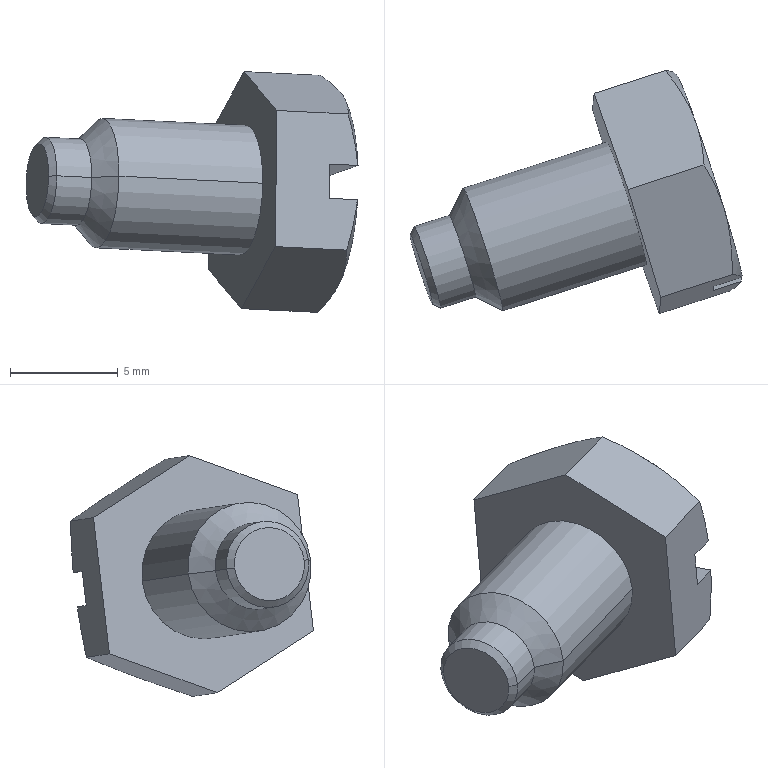Part | SolidWorks | features BaseBody 1 | 1 solid | 27 faces | box 15.373 x 11.248 x 11.146 mm | volume 566.729 mm3 | plane 13 | cone 10 | cylinder 4 | commonest cylinder face diameters 4 x2 6 x2
STEP:
#1=CARTESIAN_POINT('',(72.712,-71.322,-185.285));
#2=VERTEX_POINT('',#1);
#3=CARTESIAN_POINT('',(74.565,-76.993,-184.642));
#4=VERTEX_POINT('',#3);
#5=CARTESIAN_POINT('',(73.639,-74.158,-184.964));
#6=DIRECTION('',(0.9511,0.3055,-0.04654));
#7=DIRECTION('',(0.3088,-0.9451,0.1072));
#8=AXIS2_PLACEMENT_3D('',#5,#6,#7);
#9=CIRCLE('',#8,3.);
#10=EDGE_CURVE('',#2,#4,#9,.T.);
#11=ORIENTED_EDGE('',*,*,#10,.T.);
#12=CARTESIAN_POINT('',(81.223,-74.854,-184.968));
#13=VERTEX_POINT('',#12);
#14=CARTESIAN_POINT('',(73.614,-77.298,-184.596));
#15=DIRECTION('',(0.9511,0.3055,-0.04654));
#16=VECTOR('',#15,1000.);
#17=LINE('',#14,#16);
#18=EDGE_CURVE('',#4,#13,#17,.T.);
#19=ORIENTED_EDGE('',*,*,#18,.T.);
#20=CARTESIAN_POINT('',(79.37,-69.184,-185.611));
#21=VERTEX_POINT('',#20);
#22=CARTESIAN_POINT('',(80.296,-72.019,-185.289));
#23=DIRECTION('',(-0.9511,-0.3055,0.04654));
#24=DIRECTION('',(0.3088,-0.9451,0.1072));
#25=AXIS2_PLACEMENT_3D('',#22,#23,#24);
#26=CIRCLE('',#25,3.);
#27=EDGE_CURVE('',#13,#21,#26,.T.);
#28=ORIENTED_EDGE('',*,*,#27,.T.);
#29=CARTESIAN_POINT('',(71.761,-71.628,-185.239));
#30=DIRECTION('',(0.9511,0.3055,-0.04654));
#31=VECTOR('',#30,1000.);
#32=LINE('',#29,#31);
#33=EDGE_CURVE('',#2,#21,#32,.T.);
#34=ORIENTED_EDGE('',*,*,#33,.F.);
#35=EDGE_LOOP('',(#11,#19,#28,#34));
#36=FACE_OUTER_BOUND('',#35,.T.);
#37=CARTESIAN_POINT('',(72.688,-74.463,-184.917));
#38=DIRECTION('',(0.9511,0.3055,-0.04654));
#39=DIRECTION('',(-0.3088,0.9451,-0.1072));
#40=AXIS2_PLACEMENT_3D('',#37,#38,#39);
#41=CYLINDRICAL_SURFACE('',#40,3.);
#42=ADVANCED_FACE('',(#36),#41,.T.);
#43=CARTESIAN_POINT('',(70.453,-73.092,-185.052));
#44=VERTEX_POINT('',#43);
#45=CARTESIAN_POINT('',(71.689,-76.873,-184.624));
#46=VERTEX_POINT('',#45);
#47=CARTESIAN_POINT('',(71.071,-74.982,-184.838));
#48=DIRECTION('',(0.9511,0.3055,-0.04654));
#49=DIRECTION('',(0.3088,-0.9451,0.1072));
#50=AXIS2_PLACEMENT_3D('',#47,#48,#49);
#51=CIRCLE('',#50,2.);
#52=EDGE_CURVE('',#44,#46,#51,.T.);
#53=ORIENTED_EDGE('',*,*,#52,.T.);
#54=CARTESIAN_POINT('',(73.305,-76.353,-184.703));
#55=VERTEX_POINT('',#54);
#56=CARTESIAN_POINT('',(71.403,-76.964,-184.61));
#57=DIRECTION('',(0.9511,0.3055,-0.04654));
#58=VECTOR('',#57,1000.);
#59=LINE('',#56,#58);
#60=EDGE_CURVE('',#46,#55,#59,.T.);
#61=ORIENTED_EDGE('',*,*,#60,.T.);
#62=CARTESIAN_POINT('',(72.07,-72.573,-185.132));
#63=VERTEX_POINT('',#62);
#64=CARTESIAN_POINT('',(72.688,-74.463,-184.917));
#65=DIRECTION('',(-0.9511,-0.3055,0.04654));
#66=DIRECTION('',(0.3088,-0.9451,0.1072));
#67=AXIS2_PLACEMENT_3D('',#64,#65,#66);
#68=CIRCLE('',#67,2.);
#69=EDGE_CURVE('',#55,#63,#68,.T.);
#70=ORIENTED_EDGE('',*,*,#69,.T.);
#71=CARTESIAN_POINT('',(70.168,-73.184,-185.038));
#72=DIRECTION('',(0.9511,0.3055,-0.04654));
#73=VECTOR('',#72,1000.);
#74=LINE('',#71,#73);
#75=EDGE_CURVE('',#44,#63,#74,.T.);
#76=ORIENTED_EDGE('',*,*,#75,.F.);
#77=EDGE_LOOP('',(#53,#61,#70,#76));
#78=FACE_OUTER_BOUND('',#77,.T.);
#79=CARTESIAN_POINT('',(70.786,-75.074,-184.824));
#80=DIRECTION('',(0.9511,0.3055,-0.04654));
#81=DIRECTION('',(-0.3088,0.9451,-0.1072));
#82=AXIS2_PLACEMENT_3D('',#79,#80,#81);
#83=CYLINDRICAL_SURFACE('',#82,2.);
#84=ADVANCED_FACE('',(#78),#83,.T.);
#85=CARTESIAN_POINT('',(71.311,-76.681,-184.642));
#86=VERTEX_POINT('',#85);
#87=CARTESIAN_POINT('',(70.261,-73.467,-185.006));
#88=VERTEX_POINT('',#87);
#89=CARTESIAN_POINT('',(70.786,-75.074,-184.824));
#90=DIRECTION('',(-0.9511,-0.3055,0.04654));
#91=DIRECTION('',(0.3088,-0.9451,0.1072));
#92=AXIS2_PLACEMENT_3D('',#89,#90,#91);
#93=CIRCLE('',#92,1.7);
#94=EDGE_CURVE('',#86,#88,#93,.T.);
#95=ORIENTED_EDGE('',*,*,#94,.F.);
#96=CARTESIAN_POINT('',(71.311,-76.681,-184.642));
#97=DIRECTION('',(0.8909,-0.4522,0.04287));
#98=VECTOR('',#97,1000.);
#99=LINE('',#96,#98);
#100=EDGE_CURVE('',#86,#46,#99,.T.);
#101=ORIENTED_EDGE('',*,*,#100,.T.);
#102=ORIENTED_EDGE('',*,*,#52,.F.);
#103=CARTESIAN_POINT('',(70.261,-73.467,-185.006));
#104=DIRECTION('',(0.4541,0.8843,-0.1087));
#105=VECTOR('',#104,1000.);
#106=LINE('',#103,#105);
#107=EDGE_CURVE('',#88,#44,#106,.T.);
#108=ORIENTED_EDGE('',*,*,#107,.F.);
#109=EDGE_LOOP('',(#95,#101,#102,#108));
#110=FACE_OUTER_BOUND('',#109,.T.);
#111=CARTESIAN_POINT('',(70.786,-75.074,-184.824));
#112=DIRECTION('',(0.9511,0.3055,-0.04654));
#113=DIRECTION('',(-0.3088,0.9451,-0.1072));
#114=AXIS2_PLACEMENT_3D('',#111,#112,#113);
#115=CONICAL_SURFACE('',#114,1.7,0.7854);
#116=ADVANCED_FACE('',(#110),#115,.T.);
#117=ORIENTED_EDGE('',*,*,#69,.F.);
#118=CARTESIAN_POINT('',(73.305,-76.353,-184.703));
#119=DIRECTION('',(0.8909,-0.4522,0.04287));
#120=VECTOR('',#119,1000.);
#121=LINE('',#118,#120);
#122=EDGE_CURVE('',#55,#4,#121,.T.);
#123=ORIENTED_EDGE('',*,*,#122,.T.);
#124=ORIENTED_EDGE('',*,*,#10,.F.);
#125=CARTESIAN_POINT('',(72.07,-72.573,-185.132));
#126=DIRECTION('',(0.4541,0.8843,-0.1087));
#127=VECTOR('',#126,1000.);
#128=LINE('',#125,#127);
#129=EDGE_CURVE('',#63,#2,#128,.T.);
#130=ORIENTED_EDGE('',*,*,#129,.F.);
#131=EDGE_LOOP('',(#117,#123,#124,#130));
#132=FACE_OUTER_BOUND('',#131,.T.);
#133=CARTESIAN_POINT('',(72.688,-74.463,-184.917));
#134=DIRECTION('',(0.9511,0.3055,-0.04654));
#135=DIRECTION('',(-0.3088,0.9451,-0.1072));
#136=AXIS2_PLACEMENT_3D('',#133,#134,#135);
#137=CONICAL_SURFACE('',#136,2.,0.7854);
#138=ADVANCED_FACE('',(#132),#137,.T.);
#139=CARTESIAN_POINT('',(84.322,-75.857,-184.08));
#140=VERTEX_POINT('',#139);
#141=CARTESIAN_POINT('',(84.304,-76.043,-185.669));
#142=VERTEX_POINT('',#141);
#143=CARTESIAN_POINT('',(84.322,-75.857,-184.08));
#144=DIRECTION('',(-0.01125,-0.1163,-0.9932));
#145=VECTOR('',#144,1000.);
#146=LINE('',#143,#145);
#147=EDGE_CURVE('',#140,#142,#146,.T.);
#148=ORIENTED_EDGE('',*,*,#147,.T.);
#149=CARTESIAN_POINT('',(81.216,-66.593,-186.741));
#150=VERTEX_POINT('',#149);
#151=CARTESIAN_POINT('',(84.304,-76.043,-185.669));
#152=DIRECTION('',(-0.3088,0.9451,-0.1072));
#153=VECTOR('',#152,1000.);
#154=LINE('',#151,#153);
#155=EDGE_CURVE('',#142,#150,#154,.T.);
#156=ORIENTED_EDGE('',*,*,#155,.T.);
#157=CARTESIAN_POINT('',(81.234,-66.407,-185.152));
#158=VERTEX_POINT('',#157);
#159=CARTESIAN_POINT('',(81.216,-66.593,-186.741));
#160=DIRECTION('',(0.01125,0.1163,0.9932));
#161=VECTOR('',#160,1000.);
#162=LINE('',#159,#161);
#163=EDGE_CURVE('',#150,#158,#162,.T.);
#164=ORIENTED_EDGE('',*,*,#163,.T.);
#165=CARTESIAN_POINT('',(84.322,-75.857,-184.08));
#166=DIRECTION('',(0.3088,-0.9451,0.1072));
#167=VECTOR('',#166,1000.);
#168=LINE('',#165,#167);
#169=EDGE_CURVE('',#158,#140,#168,.T.);
#170=ORIENTED_EDGE('',*,*,#169,.T.);
#171=EDGE_LOOP('',(#148,#156,#164,#170));
#172=FACE_OUTER_BOUND('',#171,.T.);
#173=CARTESIAN_POINT('',(84.304,-76.043,-185.669));
#174=DIRECTION('',(0.9511,0.3055,-0.04654));
#175=DIRECTION('',(0.,-0.1506,-0.9886));
#176=AXIS2_PLACEMENT_3D('',#173,#174,#175);
#177=PLANE('',#176);
#178=ADVANCED_FACE('',(#172),#177,.T.);
#179=CARTESIAN_POINT('',(82.567,-66.226,-186.799));
#180=VERTEX_POINT('',#179);
#181=CARTESIAN_POINT('',(82.512,-66.176,-186.804));
#182=VERTEX_POINT('',#181);
#183=CARTESIAN_POINT('',(82.567,-66.226,-186.799));
#184=CARTESIAN_POINT('',(82.549,-66.209,-186.801));
#185=CARTESIAN_POINT('',(82.531,-66.193,-186.803));
#186=CARTESIAN_POINT('',(82.512,-66.176,-186.804));
#187=B_SPLINE_CURVE_WITH_KNOTS('',3,(#183,#184,#185,#186),.UNSPECIFIED.,.F.,.F.,(4,4),(0.,1.),.UNSPECIFIED.);
#188=EDGE_CURVE('',#180,#182,#187,.T.);
#189=ORIENTED_EDGE('',*,*,#188,.T.);
#190=CARTESIAN_POINT('',(81.216,-66.593,-186.741));
#191=DIRECTION('',(0.9511,0.3055,-0.04654));
#192=VECTOR('',#191,1000.);
#193=LINE('',#190,#192);
#194=EDGE_CURVE('',#150,#182,#193,.T.);
#195=ORIENTED_EDGE('',*,*,#194,.F.);
#196=ORIENTED_EDGE('',*,*,#155,.F.);
#197=CARTESIAN_POINT('',(85.601,-75.627,-185.733));
#198=VERTEX_POINT('',#197);
#199=CARTESIAN_POINT('',(84.304,-76.043,-185.669));
#200=DIRECTION('',(0.9511,0.3055,-0.04654));
#201=VECTOR('',#200,1000.);
#202=LINE('',#199,#201);
#203=EDGE_CURVE('',#142,#198,#202,.T.);
#204=ORIENTED_EDGE('',*,*,#203,.T.);
#205=CARTESIAN_POINT('',(85.616,-75.555,-185.741));
#206=VERTEX_POINT('',#205);
#207=CARTESIAN_POINT('',(85.601,-75.627,-185.733));
#208=CARTESIAN_POINT('',(85.605,-75.605,-185.735));
#209=CARTESIAN_POINT('',(85.61,-75.582,-185.738));
#210=CARTESIAN_POINT('',(85.615,-75.558,-185.741));
#211=CARTESIAN_POINT('',(85.615,-75.557,-185.741));
#212=CARTESIAN_POINT('',(85.616,-75.555,-185.741));
#213=B_SPLINE_CURVE_WITH_KNOTS('',3,(#207,#208,#209,#210,#211,#212),.UNSPECIFIED.,.F.,.F.,(4,2,4),(0.,0.9225,1.),.UNSPECIFIED.);
#214=EDGE_CURVE('',#198,#206,#213,.T.);
#215=ORIENTED_EDGE('',*,*,#214,.T.);
#216=CARTESIAN_POINT('',(85.635,-75.616,-185.734));
#217=DIRECTION('',(-0.3088,0.9451,-0.1072));
#218=VECTOR('',#217,1000.);
#219=LINE('',#216,#218);
#220=EDGE_CURVE('',#206,#180,#219,.T.);
#221=ORIENTED_EDGE('',*,*,#220,.T.);
#222=EDGE_LOOP('',(#189,#195,#196,#204,#215,#221));
#223=FACE_OUTER_BOUND('',#222,.T.);
#224=CARTESIAN_POINT('',(84.304,-76.043,-185.669));
#225=DIRECTION('',(-0.01125,-0.1163,-0.9932));
#226=DIRECTION('',(0.,-0.9932,0.1163));
#227=AXIS2_PLACEMENT_3D('',#224,#225,#226);
#228=PLANE('',#227);
#229=ADVANCED_FACE('',(#223),#228,.F.);
#230=CARTESIAN_POINT('',(85.634,-75.369,-184.152));
#231=VERTEX_POINT('',#230);
#232=CARTESIAN_POINT('',(85.619,-75.441,-184.144));
#233=VERTEX_POINT('',#232);
#234=CARTESIAN_POINT('',(85.634,-75.369,-184.152));
#235=CARTESIAN_POINT('',(85.629,-75.393,-184.149));
#236=CARTESIAN_POINT('',(85.624,-75.417,-184.146));
#237=CARTESIAN_POINT('',(85.619,-75.441,-184.144));
#238=B_SPLINE_CURVE_WITH_KNOTS('',3,(#234,#235,#236,#237),.UNSPECIFIED.,.F.,.F.,(4,4),(0.,1.),.UNSPECIFIED.);
#239=EDGE_CURVE('',#231,#233,#238,.T.);
#240=ORIENTED_EDGE('',*,*,#239,.T.);
#241=CARTESIAN_POINT('',(84.322,-75.857,-184.08));
#242=DIRECTION('',(0.9511,0.3055,-0.04654));
#243=VECTOR('',#242,1000.);
#244=LINE('',#241,#243);
#245=EDGE_CURVE('',#140,#233,#244,.T.);
#246=ORIENTED_EDGE('',*,*,#245,.F.);
#247=ORIENTED_EDGE('',*,*,#169,.F.);
#248=CARTESIAN_POINT('',(82.53,-65.99,-185.215));
#249=VERTEX_POINT('',#248);
#250=CARTESIAN_POINT('',(81.234,-66.407,-185.152));
#251=DIRECTION('',(0.9511,0.3055,-0.04654));
#252=VECTOR('',#251,1000.);
#253=LINE('',#250,#252);
#254=EDGE_CURVE('',#158,#249,#253,.T.);
#255=ORIENTED_EDGE('',*,*,#254,.T.);
#256=CARTESIAN_POINT('',(82.585,-66.04,-185.21));
#257=VERTEX_POINT('',#256);
#258=CARTESIAN_POINT('',(82.53,-65.99,-185.215));
#259=CARTESIAN_POINT('',(82.547,-66.005,-185.214));
#260=CARTESIAN_POINT('',(82.564,-66.021,-185.212));
#261=CARTESIAN_POINT('',(82.582,-66.037,-185.21));
#262=CARTESIAN_POINT('',(82.584,-66.038,-185.21));
#263=CARTESIAN_POINT('',(82.585,-66.04,-185.21));
#264=B_SPLINE_CURVE_WITH_KNOTS('',3,(#258,#259,#260,#261,#262,#263),.UNSPECIFIED.,.F.,.F.,(4,2,4),(0.,0.9225,1.),.UNSPECIFIED.);
#265=EDGE_CURVE('',#249,#257,#264,.T.);
#266=ORIENTED_EDGE('',*,*,#265,.T.);
#267=CARTESIAN_POINT('',(85.653,-75.43,-184.145));
#268=DIRECTION('',(0.3088,-0.9451,0.1072));
#269=VECTOR('',#268,1000.);
#270=LINE('',#267,#269);
#271=EDGE_CURVE('',#257,#231,#270,.T.);
#272=ORIENTED_EDGE('',*,*,#271,.T.);
#273=EDGE_LOOP('',(#240,#246,#247,#255,#266,#272));
#274=FACE_OUTER_BOUND('',#273,.T.);
#275=CARTESIAN_POINT('',(84.322,-75.857,-184.08));
#276=DIRECTION('',(0.01125,0.1163,0.9932));
#277=DIRECTION('',(0.9954,-0.09625,0.));
#278=AXIS2_PLACEMENT_3D('',#275,#276,#277);
#279=PLANE('',#278);
#280=ADVANCED_FACE('',(#274),#279,.F.);
#281=ORIENTED_EDGE('',*,*,#220,.F.);
#282=CARTESIAN_POINT('',(84.706,-73.334,-189.742));
#283=VERTEX_POINT('',#282);
#284=CARTESIAN_POINT('',(84.1,-70.797,-185.476));
#285=DIRECTION('',(0.9511,0.3055,-0.04654));
#286=DIRECTION('',(-0.3088,0.9451,-0.1072));
#287=AXIS2_PLACEMENT_3D('',#284,#285,#286);
#288=CIRCLE('',#287,5.);
#289=EDGE_CURVE('',#206,#283,#288,.T.);
#290=ORIENTED_EDGE('',*,*,#289,.T.);
#291=CARTESIAN_POINT('',(83.393,-69.313,-190.198));
#292=VERTEX_POINT('',#291);
#293=CARTESIAN_POINT('',(84.1,-70.797,-185.476));
#294=DIRECTION('',(0.9511,0.3055,-0.04654));
#295=DIRECTION('',(-0.3088,0.9451,-0.1072));
#296=AXIS2_PLACEMENT_3D('',#293,#294,#295);
#297=CIRCLE('',#296,5.);
#298=EDGE_CURVE('',#283,#292,#297,.T.);
#299=ORIENTED_EDGE('',*,*,#298,.T.);
#300=CARTESIAN_POINT('',(84.1,-70.797,-185.476));
#301=DIRECTION('',(0.9511,0.3055,-0.04654));
#302=DIRECTION('',(-0.3088,0.9451,-0.1072));
#303=AXIS2_PLACEMENT_3D('',#300,#301,#302);
#304=CIRCLE('',#303,5.);
#305=EDGE_CURVE('',#292,#180,#304,.T.);
#306=ORIENTED_EDGE('',*,*,#305,.T.);
#307=EDGE_LOOP('',(#281,#290,#299,#306));
#308=FACE_OUTER_BOUND('',#307,.T.);
#309=CARTESIAN_POINT('',(82.592,-65.703,-182.859));
#310=DIRECTION('',(0.9511,0.3055,-0.04654));
#311=DIRECTION('',(0.,-0.1506,-0.9886));
#312=AXIS2_PLACEMENT_3D('',#309,#310,#311);
#313=PLANE('',#312);
#314=ADVANCED_FACE('',(#308),#313,.T.);
#315=ORIENTED_EDGE('',*,*,#265,.F.);
#316=CARTESIAN_POINT('',(82.085,-65.865,-182.834));
#317=VERTEX_POINT('',#316);
#318=CARTESIAN_POINT('',(82.53,-65.99,-185.215));
#319=CARTESIAN_POINT('',(82.469,-65.918,-184.407));
#320=CARTESIAN_POINT('',(82.305,-65.882,-183.616));
#321=CARTESIAN_POINT('',(82.085,-65.865,-182.834));
#322=B_SPLINE_CURVE_WITH_KNOTS('',3,(#318,#319,#320,#321),.UNSPECIFIED.,.F.,.F.,(4,4),(0.,0.002426),.UNSPECIFIED.);
#323=EDGE_CURVE('',#249,#317,#322,.T.);
#324=ORIENTED_EDGE('',*,*,#323,.T.);
#325=CARTESIAN_POINT('',(83.494,-68.261,-181.21));
#326=VERTEX_POINT('',#325);
#327=CARTESIAN_POINT('',(82.085,-65.865,-182.834));
#328=CARTESIAN_POINT('',(82.684,-66.601,-182.312));
#329=CARTESIAN_POINT('',(83.185,-67.384,-181.775));
#330=CARTESIAN_POINT('',(83.494,-68.261,-181.21));
#331=B_SPLINE_CURVE_WITH_KNOTS('',3,(#327,#328,#329,#330),.UNSPECIFIED.,.F.,.F.,(4,4),(0.,0.003219),.UNSPECIFIED.);
#332=EDGE_CURVE('',#317,#326,#331,.T.);
#333=ORIENTED_EDGE('',*,*,#332,.T.);
#334=CARTESIAN_POINT('',(84.1,-70.797,-185.476));
#335=DIRECTION('',(0.9511,0.3055,-0.04654));
#336=DIRECTION('',(-0.3088,0.9451,-0.1072));
#337=AXIS2_PLACEMENT_3D('',#334,#335,#336);
#338=CIRCLE('',#337,5.);
#339=EDGE_CURVE('',#257,#326,#338,.T.);
#340=ORIENTED_EDGE('',*,*,#339,.F.);
#341=EDGE_LOOP('',(#315,#324,#333,#340));
#342=FACE_OUTER_BOUND('',#341,.T.);
#343=CARTESIAN_POINT('',(84.1,-70.797,-185.476));
#344=DIRECTION('',(-0.9511,-0.3055,0.04654));
#345=DIRECTION('',(-0.3088,0.9451,-0.1072));
#346=AXIS2_PLACEMENT_3D('',#343,#344,#345);
#347=CONICAL_SURFACE('',#346,5.,1.047);
#348=ADVANCED_FACE('',(#342),#347,.T.);
#349=CARTESIAN_POINT('',(83.874,-70.247,-179.974));
#350=VERTEX_POINT('',#349);
#351=CARTESIAN_POINT('',(83.494,-68.261,-181.21));
#352=CARTESIAN_POINT('',(83.721,-68.902,-180.796));
#353=CARTESIAN_POINT('',(83.835,-69.567,-180.384));
#354=CARTESIAN_POINT('',(83.874,-70.247,-179.974));
#355=B_SPLINE_CURVE_WITH_KNOTS('',3,(#351,#352,#353,#354),.UNSPECIFIED.,.F.,.F.,(4,4),(0.,0.00237),.UNSPECIFIED.);
#356=EDGE_CURVE('',#326,#350,#355,.T.);
#357=ORIENTED_EDGE('',*,*,#356,.T.);
#358=CARTESIAN_POINT('',(84.808,-72.281,-180.754));
#359=VERTEX_POINT('',#358);
#360=CARTESIAN_POINT('',(83.874,-70.247,-179.974));
#361=CARTESIAN_POINT('',(84.267,-70.888,-180.235));
#362=CARTESIAN_POINT('',(84.589,-71.561,-180.494));
#363=CARTESIAN_POINT('',(84.808,-72.281,-180.754));
#364=B_SPLINE_CURVE_WITH_KNOTS('',3,(#360,#361,#362,#363),.UNSPECIFIED.,.F.,.F.,(4,4),(0.,0.00237),.UNSPECIFIED.);
#365=EDGE_CURVE('',#350,#359,#364,.T.);
#366=ORIENTED_EDGE('',*,*,#365,.T.);
#367=CARTESIAN_POINT('',(84.1,-70.797,-185.476));
#368=DIRECTION('',(0.9511,0.3055,-0.04654));
#369=DIRECTION('',(-0.3088,0.9451,-0.1072));
#370=AXIS2_PLACEMENT_3D('',#367,#368,#369);
#371=CIRCLE('',#370,5.);
#372=EDGE_CURVE('',#326,#359,#371,.T.);
#373=ORIENTED_EDGE('',*,*,#372,.F.);
#374=EDGE_LOOP('',(#357,#366,#373));
#375=FACE_OUTER_BOUND('',#374,.T.);
#376=CARTESIAN_POINT('',(84.1,-70.797,-185.476));
#377=DIRECTION('',(-0.9511,-0.3055,0.04654));
#378=DIRECTION('',(-0.3088,0.9451,-0.1072));
#379=AXIS2_PLACEMENT_3D('',#376,#377,#378);
#380=CONICAL_SURFACE('',#379,5.,1.047);
#381=ADVANCED_FACE('',(#375),#380,.T.);
#382=ORIENTED_EDGE('',*,*,#239,.F.);
#383=CARTESIAN_POINT('',(84.1,-70.797,-185.476));
#384=DIRECTION('',(0.9511,0.3055,-0.04654));
#385=DIRECTION('',(-0.3088,0.9451,-0.1072));
#386=AXIS2_PLACEMENT_3D('',#383,#384,#385);
#387=CIRCLE('',#386,5.);
#388=EDGE_CURVE('',#359,#231,#387,.T.);
#389=ORIENTED_EDGE('',*,*,#388,.F.);
#390=CARTESIAN_POINT('',(85.174,-75.316,-181.762));
#391=VERTEX_POINT('',#390);
#392=CARTESIAN_POINT('',(84.808,-72.281,-180.754));
#393=CARTESIAN_POINT('',(85.107,-73.266,-181.108));
#394=CARTESIAN_POINT('',(85.194,-74.283,-181.441));
#395=CARTESIAN_POINT('',(85.174,-75.316,-181.762));
#396=B_SPLINE_CURVE_WITH_KNOTS('',3,(#392,#393,#394,#395),.UNSPECIFIED.,.F.,.F.,(4,4),(0.,0.003219),.UNSPECIFIED.);
#397=EDGE_CURVE('',#359,#391,#396,.T.);
#398=ORIENTED_EDGE('',*,*,#397,.T.);
#399=CARTESIAN_POINT('',(85.174,-75.316,-181.762));
#400=CARTESIAN_POINT('',(85.393,-75.333,-182.544));
#401=CARTESIAN_POINT('',(85.557,-75.369,-183.335));
#402=CARTESIAN_POINT('',(85.619,-75.441,-184.144));
#403=B_SPLINE_CURVE_WITH_KNOTS('',3,(#399,#400,#401,#402),.UNSPECIFIED.,.F.,.F.,(4,4),(0.,0.002426),.UNSPECIFIED.);
#404=EDGE_CURVE('',#391,#233,#403,.T.);
#405=ORIENTED_EDGE('',*,*,#404,.T.);
#406=EDGE_LOOP('',(#382,#389,#398,#405));
#407=FACE_OUTER_BOUND('',#406,.T.);
#408=CARTESIAN_POINT('',(84.1,-70.797,-185.476));
#409=DIRECTION('',(-0.9511,-0.3055,0.04654));
#410=DIRECTION('',(-0.3088,0.9451,-0.1072));
#411=AXIS2_PLACEMENT_3D('',#408,#409,#410);
#412=CONICAL_SURFACE('',#411,5.,1.047);
#413=ADVANCED_FACE('',(#407),#412,.T.);
#414=ORIENTED_EDGE('',*,*,#214,.F.);
#415=CARTESIAN_POINT('',(85.102,-76.054,-188.068));
#416=VERTEX_POINT('',#415);
#417=CARTESIAN_POINT('',(85.601,-75.627,-185.733));
#418=CARTESIAN_POINT('',(85.521,-75.744,-186.534));
#419=CARTESIAN_POINT('',(85.339,-75.891,-187.308));
#420=CARTESIAN_POINT('',(85.102,-76.054,-188.068));
#421=B_SPLINE_CURVE_WITH_KNOTS('',3,(#417,#418,#419,#420),.UNSPECIFIED.,.F.,.F.,(4,4),(0.,0.002426),.UNSPECIFIED.);
#422=EDGE_CURVE('',#198,#416,#421,.T.);
#423=ORIENTED_EDGE('',*,*,#422,.T.);
#424=CARTESIAN_POINT('',(85.102,-76.054,-188.068));
#425=CARTESIAN_POINT('',(85.113,-75.123,-188.62));
#426=CARTESIAN_POINT('',(85.016,-74.21,-189.176));
#427=CARTESIAN_POINT('',(84.706,-73.334,-189.742));
#428=B_SPLINE_CURVE_WITH_KNOTS('',3,(#424,#425,#426,#427),.UNSPECIFIED.,.F.,.F.,(4,4),(0.,0.003219),.UNSPECIFIED.);
#429=EDGE_CURVE('',#416,#283,#428,.T.);
#430=ORIENTED_EDGE('',*,*,#429,.T.);
#431=ORIENTED_EDGE('',*,*,#289,.F.);
#432=EDGE_LOOP('',(#414,#423,#430,#431));
#433=FACE_OUTER_BOUND('',#432,.T.);
#434=CARTESIAN_POINT('',(84.1,-70.797,-185.476));
#435=DIRECTION('',(-0.9511,-0.3055,0.04654));
#436=DIRECTION('',(-0.3088,0.9451,-0.1072));
#437=AXIS2_PLACEMENT_3D('',#434,#435,#436);
#438=CONICAL_SURFACE('',#437,5.,1.047);
#439=ADVANCED_FACE('',(#433),#438,.T.);
#440=CARTESIAN_POINT('',(83.75,-71.532,-190.949));
#441=VERTEX_POINT('',#440);
#442=CARTESIAN_POINT('',(83.75,-71.532,-190.949));
#443=CARTESIAN_POINT('',(83.718,-70.776,-190.706));
#444=CARTESIAN_POINT('',(83.611,-70.034,-190.457));
#445=CARTESIAN_POINT('',(83.393,-69.313,-190.198));
#446=B_SPLINE_CURVE_WITH_KNOTS('',3,(#442,#443,#444,#445),.UNSPECIFIED.,.F.,.F.,(4,4),(0.,0.00237),.UNSPECIFIED.);
#447=EDGE_CURVE('',#441,#292,#446,.T.);
#448=ORIENTED_EDGE('',*,*,#447,.T.);
#449=ORIENTED_EDGE('',*,*,#298,.F.);
#450=CARTESIAN_POINT('',(84.706,-73.334,-189.742));
#451=CARTESIAN_POINT('',(84.48,-72.692,-190.155));
#452=CARTESIAN_POINT('',(84.15,-72.097,-190.556));
#453=CARTESIAN_POINT('',(83.75,-71.532,-190.949));
#454=B_SPLINE_CURVE_WITH_KNOTS('',3,(#450,#451,#452,#453),.UNSPECIFIED.,.F.,.F.,(4,4),(0.,0.00237),.UNSPECIFIED.);
#455=EDGE_CURVE('',#283,#441,#454,.T.);
#456=ORIENTED_EDGE('',*,*,#455,.T.);
#457=EDGE_LOOP('',(#448,#449,#456));
#458=FACE_OUTER_BOUND('',#457,.T.);
#459=CARTESIAN_POINT('',(84.1,-70.797,-185.476));
#460=DIRECTION('',(-0.9511,-0.3055,0.04654));
#461=DIRECTION('',(-0.3088,0.9451,-0.1072));
#462=AXIS2_PLACEMENT_3D('',#459,#460,#461);
#463=CONICAL_SURFACE('',#462,5.,1.047);
#464=ADVANCED_FACE('',(#458),#463,.T.);
#465=ORIENTED_EDGE('',*,*,#188,.F.);
#466=ORIENTED_EDGE('',*,*,#305,.F.);
#467=CARTESIAN_POINT('',(82.014,-66.604,-189.139));
#468=VERTEX_POINT('',#467);
#469=CARTESIAN_POINT('',(83.393,-69.313,-190.198));
#470=CARTESIAN_POINT('',(83.094,-68.329,-189.843));
#471=CARTESIAN_POINT('',(82.603,-67.442,-189.491));
#472=CARTESIAN_POINT('',(82.014,-66.604,-189.139));
#473=B_SPLINE_CURVE_WITH_KNOTS('',3,(#469,#470,#471,#472),.UNSPECIFIED.,.F.,.F.,(4,4),(0.,0.003219),.UNSPECIFIED.);
#474=EDGE_CURVE('',#292,#468,#473,.T.);
#475=ORIENTED_EDGE('',*,*,#474,.T.);
#476=CARTESIAN_POINT('',(82.014,-66.604,-189.139));
#477=CARTESIAN_POINT('',(82.251,-66.44,-188.38));
#478=CARTESIAN_POINT('',(82.433,-66.293,-187.606));
#479=CARTESIAN_POINT('',(82.512,-66.176,-186.804));
#480=B_SPLINE_CURVE_WITH_KNOTS('',3,(#476,#477,#478,#479),.UNSPECIFIED.,.F.,.F.,(4,4),(0.,0.002426),.UNSPECIFIED.);
#481=EDGE_CURVE('',#468,#182,#480,.T.);
#482=ORIENTED_EDGE('',*,*,#481,.T.);
#483=EDGE_LOOP('',(#465,#466,#475,#482));
#484=FACE_OUTER_BOUND('',#483,.T.);
#485=CARTESIAN_POINT('',(84.1,-70.797,-185.476));
#486=DIRECTION('',(-0.9511,-0.3055,0.04654));
#487=DIRECTION('',(-0.3088,0.9451,-0.1072));
#488=AXIS2_PLACEMENT_3D('',#485,#486,#487);
#489=CONICAL_SURFACE('',#488,5.,1.047);
#490=ADVANCED_FACE('',(#484),#489,.T.);
#491=ORIENTED_EDGE('',*,*,#122,.F.);
#492=CARTESIAN_POINT('',(72.688,-74.463,-184.917));
#493=DIRECTION('',(-0.9511,-0.3055,0.04654));
#494=DIRECTION('',(0.3088,-0.9451,0.1072));
#495=AXIS2_PLACEMENT_3D('',#492,#493,#494);
#496=CIRCLE('',#495,2.);
#497=EDGE_CURVE('',#63,#55,#496,.T.);
#498=ORIENTED_EDGE('',*,*,#497,.F.);
#499=ORIENTED_EDGE('',*,*,#129,.T.);
#500=CARTESIAN_POINT('',(73.639,-74.158,-184.964));
#501=DIRECTION('',(0.9511,0.3055,-0.04654));
#502=DIRECTION('',(0.3088,-0.9451,0.1072));
#503=AXIS2_PLACEMENT_3D('',#500,#501,#502);
#504=CIRCLE('',#503,3.);
#505=EDGE_CURVE('',#4,#2,#504,.T.);
#506=ORIENTED_EDGE('',*,*,#505,.F.);
#507=EDGE_LOOP('',(#491,#498,#499,#506));
#508=FACE_OUTER_BOUND('',#507,.T.);
#509=CARTESIAN_POINT('',(72.688,-74.463,-184.917));
#510=DIRECTION('',(0.9511,0.3055,-0.04654));
#511=DIRECTION('',(-0.3088,0.9451,-0.1072));
#512=AXIS2_PLACEMENT_3D('',#509,#510,#511);
#513=CONICAL_SURFACE('',#512,2.,0.7854);
#514=ADVANCED_FACE('',(#508),#513,.T.);
#515=ORIENTED_EDGE('',*,*,#100,.F.);
#516=CARTESIAN_POINT('',(70.786,-75.074,-184.824));
#517=DIRECTION('',(-0.9511,-0.3055,0.04654));
#518=DIRECTION('',(0.3088,-0.9451,0.1072));
#519=AXIS2_PLACEMENT_3D('',#516,#517,#518);
#520=CIRCLE('',#519,1.7);
#521=EDGE_CURVE('',#88,#86,#520,.T.);
#522=ORIENTED_EDGE('',*,*,#521,.F.);
#523=ORIENTED_EDGE('',*,*,#107,.T.);
#524=CARTESIAN_POINT('',(71.071,-74.982,-184.838));
#525=DIRECTION('',(0.9511,0.3055,-0.04654));
#526=DIRECTION('',(0.3088,-0.9451,0.1072));
#527=AXIS2_PLACEMENT_3D('',#524,#525,#526);
#528=CIRCLE('',#527,2.);
#529=EDGE_CURVE('',#46,#44,#528,.T.);
#530=ORIENTED_EDGE('',*,*,#529,.F.);
#531=EDGE_LOOP('',(#515,#522,#523,#530));
#532=FACE_OUTER_BOUND('',#531,.T.);
#533=CARTESIAN_POINT('',(70.786,-75.074,-184.824));
#534=DIRECTION('',(0.9511,0.3055,-0.04654));
#535=DIRECTION('',(-0.3088,0.9451,-0.1072));
#536=AXIS2_PLACEMENT_3D('',#533,#534,#535);
#537=CONICAL_SURFACE('',#536,1.7,0.7854);
#538=ADVANCED_FACE('',(#532),#537,.T.);
#539=ORIENTED_EDGE('',*,*,#521,.T.);
#540=ORIENTED_EDGE('',*,*,#94,.T.);
#541=EDGE_LOOP('',(#539,#540));
#542=FACE_OUTER_BOUND('',#541,.T.);
#543=CARTESIAN_POINT('',(70.786,-75.074,-184.824));
#544=DIRECTION('',(-0.9511,-0.3055,0.04654));
#545=DIRECTION('',(-0.3058,0.9521,0.));
#546=AXIS2_PLACEMENT_3D('',#543,#544,#545);
#547=PLANE('',#546);
#548=ADVANCED_FACE('',(#542),#547,.T.);
#549=ORIENTED_EDGE('',*,*,#60,.F.);
#550=ORIENTED_EDGE('',*,*,#529,.T.);
#551=ORIENTED_EDGE('',*,*,#75,.T.);
#552=ORIENTED_EDGE('',*,*,#497,.T.);
#553=EDGE_LOOP('',(#549,#550,#551,#552));
#554=FACE_OUTER_BOUND('',#553,.T.);
#555=CARTESIAN_POINT('',(70.786,-75.074,-184.824));
#556=DIRECTION('',(0.9511,0.3055,-0.04654));
#557=DIRECTION('',(-0.3088,0.9451,-0.1072));
#558=AXIS2_PLACEMENT_3D('',#555,#556,#557);
#559=CYLINDRICAL_SURFACE('',#558,2.);
#560=ADVANCED_FACE('',(#554),#559,.T.);
#561=ORIENTED_EDGE('',*,*,#18,.F.);
#562=ORIENTED_EDGE('',*,*,#505,.T.);
#563=ORIENTED_EDGE('',*,*,#33,.T.);
#564=CARTESIAN_POINT('',(80.296,-72.019,-185.289));
#565=DIRECTION('',(-0.9511,-0.3055,0.04654));
#566=DIRECTION('',(0.3088,-0.9451,0.1072));
#567=AXIS2_PLACEMENT_3D('',#564,#565,#566);
#568=CIRCLE('',#567,3.);
#569=EDGE_CURVE('',#21,#13,#568,.T.);
#570=ORIENTED_EDGE('',*,*,#569,.T.);
#571=EDGE_LOOP('',(#561,#562,#563,#570));
#572=FACE_OUTER_BOUND('',#571,.T.);
#573=CARTESIAN_POINT('',(72.688,-74.463,-184.917));
#574=DIRECTION('',(0.9511,0.3055,-0.04654));
#575=DIRECTION('',(-0.3088,0.9451,-0.1072));
#576=AXIS2_PLACEMENT_3D('',#573,#574,#575);
#577=CYLINDRICAL_SURFACE('',#576,3.);
#578=ADVANCED_FACE('',(#572),#577,.T.);
#579=ORIENTED_EDGE('',*,*,#569,.F.);
#580=ORIENTED_EDGE('',*,*,#27,.F.);
#581=EDGE_LOOP('',(#579,#580));
#582=FACE_BOUND('',#581,.T.);
#583=CARTESIAN_POINT('',(80.358,-71.377,-179.802));
#584=VERTEX_POINT('',#583);
#585=CARTESIAN_POINT('',(78.788,-66.925,-182.673));
#586=VERTEX_POINT('',#585);
#587=CARTESIAN_POINT('',(80.358,-71.377,-179.802));
#588=DIRECTION('',(-0.2843,0.8058,-0.5195));
#589=VECTOR('',#588,1000.);
#590=LINE('',#587,#589);
#591=EDGE_CURVE('',#584,#586,#590,.T.);
#592=ORIENTED_EDGE('',*,*,#591,.T.);
#593=CARTESIAN_POINT('',(78.716,-67.663,-188.978));
#594=VERTEX_POINT('',#593);
#595=CARTESIAN_POINT('',(78.716,-67.663,-188.978));
#596=DIRECTION('',(-0.01125,-0.1163,-0.9932));
#597=VECTOR('',#596,1000.);
#598=LINE('',#595,#597);
#599=EDGE_CURVE('',#586,#594,#598,.T.);
#600=ORIENTED_EDGE('',*,*,#599,.T.);
#601=CARTESIAN_POINT('',(80.234,-72.662,-190.777));
#602=VERTEX_POINT('',#601);
#603=CARTESIAN_POINT('',(80.234,-72.662,-190.777));
#604=DIRECTION('',(0.2747,-0.9047,-0.3256));
#605=VECTOR('',#604,1000.);
#606=LINE('',#603,#605);
#607=EDGE_CURVE('',#594,#602,#606,.T.);
#608=ORIENTED_EDGE('',*,*,#607,.T.);
#609=CARTESIAN_POINT('',(81.805,-77.114,-187.906));
#610=VERTEX_POINT('',#609);
#611=CARTESIAN_POINT('',(80.234,-72.662,-190.777));
#612=DIRECTION('',(0.2843,-0.8058,0.5195));
#613=VECTOR('',#612,1000.);
#614=LINE('',#611,#613);
#615=EDGE_CURVE('',#602,#610,#614,.T.);
#616=ORIENTED_EDGE('',*,*,#615,.T.);
#617=CARTESIAN_POINT('',(81.876,-76.375,-181.601));
#618=VERTEX_POINT('',#617);
#619=CARTESIAN_POINT('',(81.805,-77.114,-187.906));
#620=DIRECTION('',(0.01125,0.1163,0.9932));
#621=VECTOR('',#620,1000.);
#622=LINE('',#619,#621);
#623=EDGE_CURVE('',#610,#618,#622,.T.);
#624=ORIENTED_EDGE('',*,*,#623,.T.);
#625=CARTESIAN_POINT('',(80.358,-71.377,-179.802));
#626=DIRECTION('',(-0.2747,0.9047,0.3256));
#627=VECTOR('',#626,1000.);
#628=LINE('',#625,#627);
#629=EDGE_CURVE('',#618,#584,#628,.T.);
#630=ORIENTED_EDGE('',*,*,#629,.T.);
#631=EDGE_LOOP('',(#592,#600,#608,#616,#624,#630));
#632=FACE_OUTER_BOUND('',#631,.T.);
#633=CARTESIAN_POINT('',(78.788,-66.925,-182.673));
#634=DIRECTION('',(0.9511,0.3055,-0.04654));
#635=DIRECTION('',(0.,-0.1506,-0.9886));
#636=AXIS2_PLACEMENT_3D('',#633,#634,#635);
#637=PLANE('',#636);
#638=ADVANCED_FACE('',(#582,#632),#637,.F.);
#639=ORIENTED_EDGE('',*,*,#365,.F.);
#640=CARTESIAN_POINT('',(80.358,-71.377,-179.802));
#641=DIRECTION('',(0.9511,0.3055,-0.04654));
#642=VECTOR('',#641,1000.);
#643=LINE('',#640,#642);
#644=EDGE_CURVE('',#584,#350,#643,.T.);
#645=ORIENTED_EDGE('',*,*,#644,.F.);
#646=ORIENTED_EDGE('',*,*,#629,.F.);
#647=CARTESIAN_POINT('',(81.876,-76.375,-181.601));
#648=DIRECTION('',(0.9511,0.3055,-0.04654));
#649=VECTOR('',#648,1000.);
#650=LINE('',#647,#649);
#651=EDGE_CURVE('',#618,#391,#650,.T.);
#652=ORIENTED_EDGE('',*,*,#651,.T.);
#653=ORIENTED_EDGE('',*,*,#397,.F.);
#654=EDGE_LOOP('',(#639,#645,#646,#652,#653));
#655=FACE_OUTER_BOUND('',#654,.T.);
#656=CARTESIAN_POINT('',(80.358,-71.377,-179.802));
#657=DIRECTION('',(-0.1416,0.2968,-0.9444));
#658=DIRECTION('',(-0.989,0.,0.1482));
#659=AXIS2_PLACEMENT_3D('',#656,#657,#658);
#660=PLANE('',#659);
#661=ADVANCED_FACE('',(#655),#660,.F.);
#662=ORIENTED_EDGE('',*,*,#147,.F.);
#663=ORIENTED_EDGE('',*,*,#245,.T.);
#664=ORIENTED_EDGE('',*,*,#404,.F.);
#665=ORIENTED_EDGE('',*,*,#651,.F.);
#666=ORIENTED_EDGE('',*,*,#623,.F.);
#667=CARTESIAN_POINT('',(81.805,-77.114,-187.906));
#668=DIRECTION('',(0.9511,0.3055,-0.04654));
#669=VECTOR('',#668,1000.);
#670=LINE('',#667,#669);
#671=EDGE_CURVE('',#610,#416,#670,.T.);
#672=ORIENTED_EDGE('',*,*,#671,.T.);
#673=ORIENTED_EDGE('',*,*,#422,.F.);
#674=ORIENTED_EDGE('',*,*,#203,.F.);
#675=EDGE_LOOP('',(#662,#663,#664,#665,#666,#672,#673,#674));
#676=FACE_OUTER_BOUND('',#675,.T.);
#677=CARTESIAN_POINT('',(81.805,-77.114,-187.906));
#678=DIRECTION('',(-0.3088,0.9451,-0.1072));
#679=DIRECTION('',(-0.3278,0.,0.9447));
#680=AXIS2_PLACEMENT_3D('',#677,#678,#679);
#681=PLANE('',#680);
#682=ADVANCED_FACE('',(#676),#681,.F.);
#683=ORIENTED_EDGE('',*,*,#429,.F.);
#684=ORIENTED_EDGE('',*,*,#671,.F.);
#685=ORIENTED_EDGE('',*,*,#615,.F.);
#686=CARTESIAN_POINT('',(80.234,-72.662,-190.777));
#687=DIRECTION('',(0.9511,0.3055,-0.04654));
#688=VECTOR('',#687,1000.);
#689=LINE('',#686,#688);
#690=EDGE_CURVE('',#602,#441,#689,.T.);
#691=ORIENTED_EDGE('',*,*,#690,.T.);
#692=ORIENTED_EDGE('',*,*,#455,.F.);
#693=EDGE_LOOP('',(#683,#684,#685,#691,#692));
#694=FACE_OUTER_BOUND('',#693,.T.);
#695=CARTESIAN_POINT('',(80.234,-72.662,-190.777));
#696=DIRECTION('',(-0.1212,0.5073,0.8532));
#697=DIRECTION('',(0.9726,0.2324,0.));
#698=AXIS2_PLACEMENT_3D('',#695,#696,#697);
#699=PLANE('',#698);
#700=ADVANCED_FACE('',(#694),#699,.F.);
#701=ORIENTED_EDGE('',*,*,#447,.F.);
#702=ORIENTED_EDGE('',*,*,#690,.F.);
#703=ORIENTED_EDGE('',*,*,#607,.F.);
#704=CARTESIAN_POINT('',(78.716,-67.663,-188.978));
#705=DIRECTION('',(0.9511,0.3055,-0.04654));
#706=VECTOR('',#705,1000.);
#707=LINE('',#704,#706);
#708=EDGE_CURVE('',#594,#468,#707,.T.);
#709=ORIENTED_EDGE('',*,*,#708,.T.);
#710=ORIENTED_EDGE('',*,*,#474,.F.);
#711=EDGE_LOOP('',(#701,#702,#703,#709,#710));
#712=FACE_OUTER_BOUND('',#711,.T.);
#713=CARTESIAN_POINT('',(80.234,-72.662,-190.777));
#714=DIRECTION('',(0.1416,-0.2968,0.9444));
#715=DIRECTION('',(-0.9026,-0.4304,0.));
#716=AXIS2_PLACEMENT_3D('',#713,#714,#715);
#717=PLANE('',#716);
#718=ADVANCED_FACE('',(#712),#717,.F.);
#719=ORIENTED_EDGE('',*,*,#323,.F.);
#720=ORIENTED_EDGE('',*,*,#254,.F.);
#721=ORIENTED_EDGE('',*,*,#163,.F.);
#722=ORIENTED_EDGE('',*,*,#194,.T.);
#723=ORIENTED_EDGE('',*,*,#481,.F.);
#724=ORIENTED_EDGE('',*,*,#708,.F.);
#725=ORIENTED_EDGE('',*,*,#599,.F.);
#726=CARTESIAN_POINT('',(78.788,-66.925,-182.673));
#727=DIRECTION('',(0.9511,0.3055,-0.04654));
#728=VECTOR('',#727,1000.);
#729=LINE('',#726,#728);
#730=EDGE_CURVE('',#586,#317,#729,.T.);
#731=ORIENTED_EDGE('',*,*,#730,.T.);
#732=EDGE_LOOP('',(#719,#720,#721,#722,#723,#724,#725,#731));
#733=FACE_OUTER_BOUND('',#732,.T.);
#734=CARTESIAN_POINT('',(78.716,-67.663,-188.978));
#735=DIRECTION('',(0.3088,-0.9451,0.1072));
#736=DIRECTION('',(0.,-0.1127,-0.9936));
#737=AXIS2_PLACEMENT_3D('',#734,#735,#736);
#738=PLANE('',#737);
#739=ADVANCED_FACE('',(#733),#738,.F.);
#740=ORIENTED_EDGE('',*,*,#332,.F.);
#741=ORIENTED_EDGE('',*,*,#730,.F.);
#742=ORIENTED_EDGE('',*,*,#591,.F.);
#743=ORIENTED_EDGE('',*,*,#644,.T.);
#744=ORIENTED_EDGE('',*,*,#356,.F.);
#745=EDGE_LOOP('',(#740,#741,#742,#743,#744));
#746=FACE_OUTER_BOUND('',#745,.T.);
#747=CARTESIAN_POINT('',(80.358,-71.377,-179.802));
#748=DIRECTION('',(0.1212,-0.5073,-0.8532));
#749=DIRECTION('',(0.,-0.8595,0.5111));
#750=AXIS2_PLACEMENT_3D('',#747,#748,#749);
#751=PLANE('',#750);
#752=ADVANCED_FACE('',(#746),#751,.F.);
#753=ORIENTED_EDGE('',*,*,#271,.F.);
#754=ORIENTED_EDGE('',*,*,#339,.T.);
#755=ORIENTED_EDGE('',*,*,#372,.T.);
#756=ORIENTED_EDGE('',*,*,#388,.T.);
#757=EDGE_LOOP('',(#753,#754,#755,#756));
#758=FACE_OUTER_BOUND('',#757,.T.);
#759=CARTESIAN_POINT('',(82.592,-65.703,-182.859));
#760=DIRECTION('',(0.9511,0.3055,-0.04654));
#761=DIRECTION('',(0.,-0.1506,-0.9886));
#762=AXIS2_PLACEMENT_3D('',#759,#760,#761);
#763=PLANE('',#762);
#764=ADVANCED_FACE('',(#758),#763,.T.);
#765=CLOSED_SHELL('',(#42,#84,#116,#138,#178,#229,#280,#314,#348,#381,#413,#439,#464,#490,#514,#538,#548,#560,#578,#638,#661,#682,#700,#718,#739,#752,#764));
#766=MANIFOLD_SOLID_BREP('',#765);
#767=CARTESIAN_POINT('',(0.,0.,0.));
#768=DIRECTION('',(0.,0.,1.));
#769=DIRECTION('',(1.,0.,0.));
#770=AXIS2_PLACEMENT_3D('',#767,#768,#769);
#771=(LENGTH_UNIT()NAMED_UNIT(*)SI_UNIT(.MILLI.,.METRE.));
#772=UNCERTAINTY_MEASURE_WITH_UNIT(LENGTH_MEASURE(0.00001),#771,'','');
#773=(NAMED_UNIT(*)PLANE_ANGLE_UNIT()SI_UNIT($,.RADIAN.));
#774=(NAMED_UNIT(*)SI_UNIT($,.STERADIAN.)SOLID_ANGLE_UNIT());
#775=(GEOMETRIC_REPRESENTATION_CONTEXT(3)GLOBAL_UNCERTAINTY_ASSIGNED_CONTEXT((#772))GLOBAL_UNIT_ASSIGNED_CONTEXT((#771,#773,#774))REPRESENTATION_CONTEXT('',''));
#776=ADVANCED_BREP_SHAPE_REPRESENTATION('',(#766,#770),#775);